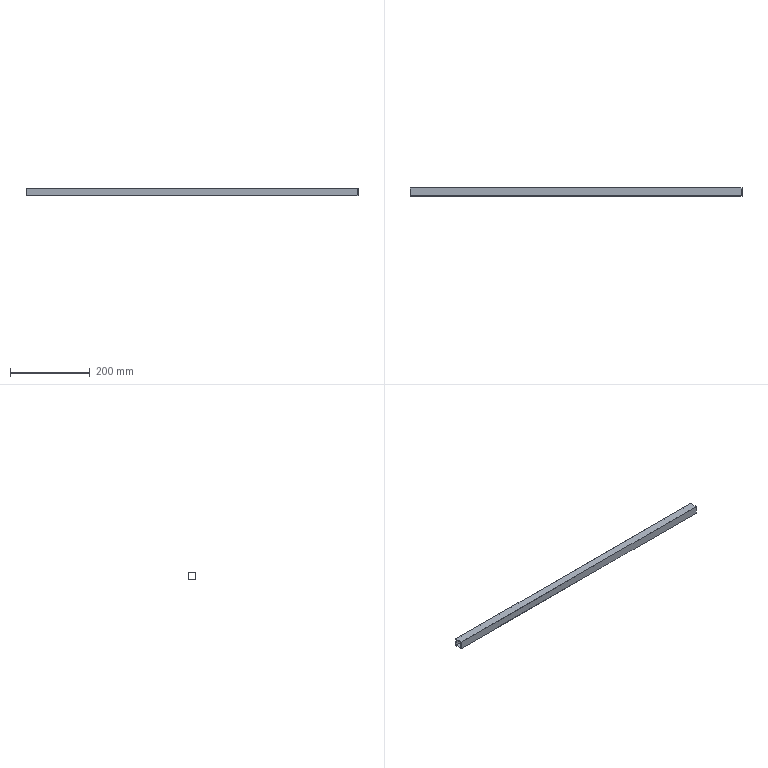Part | NX | features BREP 1 | 1 solid | 10 faces | box 830.914 x 20 x 20 mm | volume 119652 mm3 | plane 10
STEP:
#1=CARTESIAN_POINT('',(1608.587,-696.,89.999));
#2=VERTEX_POINT('',#1);
#3=CARTESIAN_POINT('',(1608.587,-680.,89.999));
#4=VERTEX_POINT('',#3);
#5=CARTESIAN_POINT('',(1608.587,-688.,89.999));
#6=DIRECTION('',(0.,1.,0.));
#7=VECTOR('',#6,1000.);
#8=LINE('',#5,#7);
#9=EDGE_CURVE('',#2,#4,#8,.T.);
#10=ORIENTED_EDGE('',*,*,#9,.F.);
#11=CARTESIAN_POINT('',(1608.587,-696.,105.999));
#12=VERTEX_POINT('',#11);
#13=CARTESIAN_POINT('',(1608.587,-696.,97.999));
#14=DIRECTION('',(0.,0.,1.));
#15=VECTOR('',#14,1000.);
#16=LINE('',#13,#15);
#17=EDGE_CURVE('',#2,#12,#16,.T.);
#18=ORIENTED_EDGE('',*,*,#17,.T.);
#19=CARTESIAN_POINT('',(1608.587,-680.,105.999));
#20=VERTEX_POINT('',#19);
#21=CARTESIAN_POINT('',(1608.587,-688.,105.999));
#22=DIRECTION('',(0.,-1.,0.));
#23=VECTOR('',#22,1000.);
#24=LINE('',#21,#23);
#25=EDGE_CURVE('',#20,#12,#24,.T.);
#26=ORIENTED_EDGE('',*,*,#25,.F.);
#27=CARTESIAN_POINT('',(1608.587,-680.,97.999));
#28=DIRECTION('',(0.,0.,1.));
#29=VECTOR('',#28,1000.);
#30=LINE('',#27,#29);
#31=EDGE_CURVE('',#4,#20,#30,.T.);
#32=ORIENTED_EDGE('',*,*,#31,.F.);
#33=EDGE_LOOP('',(#10,#18,#26,#32));
#34=FACE_BOUND('',#33,.T.);
#35=CARTESIAN_POINT('',(1608.587,-698.,87.999));
#36=VERTEX_POINT('',#35);
#37=CARTESIAN_POINT('',(1608.587,-698.,107.999));
#38=VERTEX_POINT('',#37);
#39=CARTESIAN_POINT('',(1608.587,-698.,87.999));
#40=CARTESIAN_POINT('',(1608.587,-698.,107.999));
#41=B_SPLINE_CURVE_WITH_KNOTS('',1,(#39,#40),.UNSPECIFIED.,.F.,.F.,(2,2),(0.,20.),.UNSPECIFIED.);
#42=EDGE_CURVE('',#36,#38,#41,.T.);
#43=ORIENTED_EDGE('',*,*,#42,.F.);
#44=CARTESIAN_POINT('',(1608.587,-678.,87.999));
#45=VERTEX_POINT('',#44);
#46=CARTESIAN_POINT('',(1608.587,-688.,87.999));
#47=DIRECTION('',(0.,1.,0.));
#48=VECTOR('',#47,1000.);
#49=LINE('',#46,#48);
#50=EDGE_CURVE('',#36,#45,#49,.T.);
#51=ORIENTED_EDGE('',*,*,#50,.T.);
#52=CARTESIAN_POINT('',(1608.587,-678.,107.999));
#53=VERTEX_POINT('',#52);
#54=CARTESIAN_POINT('',(1608.587,-678.,97.999));
#55=DIRECTION('',(0.,0.,1.));
#56=VECTOR('',#55,1000.);
#57=LINE('',#54,#56);
#58=EDGE_CURVE('',#45,#53,#57,.T.);
#59=ORIENTED_EDGE('',*,*,#58,.T.);
#60=CARTESIAN_POINT('',(1608.587,-688.,107.999));
#61=DIRECTION('',(0.,-1.,0.));
#62=VECTOR('',#61,1000.);
#63=LINE('',#60,#62);
#64=EDGE_CURVE('',#53,#38,#63,.T.);
#65=ORIENTED_EDGE('',*,*,#64,.T.);
#66=EDGE_LOOP('',(#43,#51,#59,#65));
#67=FACE_BOUND('',#66,.T.);
#68=CARTESIAN_POINT('',(1608.587,-688.,659.408));
#69=DIRECTION('',(1.,0.,0.));
#70=DIRECTION('',(0.,0.,-1.));
#71=AXIS2_PLACEMENT_3D('',#68,#69,#70);
#72=PLANE('',#71);
#73=ADVANCED_FACE('',(#34,#67),#72,.T.);
#74=CARTESIAN_POINT('',(777.673,-680.,105.999));
#75=VERTEX_POINT('',#74);
#76=CARTESIAN_POINT('',(1193.13,-680.,105.999));
#77=DIRECTION('',(1.,0.,0.));
#78=VECTOR('',#77,1000.);
#79=LINE('',#76,#78);
#80=EDGE_CURVE('',#75,#20,#79,.T.);
#81=ORIENTED_EDGE('',*,*,#80,.F.);
#82=CARTESIAN_POINT('',(777.673,-680.,89.999));
#83=VERTEX_POINT('',#82);
#84=CARTESIAN_POINT('',(777.673,-680.,89.999));
#85=CARTESIAN_POINT('',(777.673,-680.,93.199));
#86=CARTESIAN_POINT('',(777.673,-680.,96.399));
#87=CARTESIAN_POINT('',(777.673,-680.,99.599));
#88=CARTESIAN_POINT('',(777.673,-680.,102.799));
#89=CARTESIAN_POINT('',(777.673,-680.,105.999));
#90=B_SPLINE_CURVE_WITH_KNOTS('',5,(#84,#85,#86,#87,#88,#89),.UNSPECIFIED.,.F.,.F.,(6,6),(-286.004,-270.004),.UNSPECIFIED.);
#91=EDGE_CURVE('',#83,#75,#90,.T.);
#92=ORIENTED_EDGE('',*,*,#91,.F.);
#93=CARTESIAN_POINT('',(1193.13,-680.,89.999));
#94=DIRECTION('',(1.,0.,0.));
#95=VECTOR('',#94,1000.);
#96=LINE('',#93,#95);
#97=EDGE_CURVE('',#83,#4,#96,.T.);
#98=ORIENTED_EDGE('',*,*,#97,.T.);
#99=ORIENTED_EDGE('',*,*,#31,.T.);
#100=EDGE_LOOP('',(#81,#92,#98,#99));
#101=FACE_BOUND('',#100,.T.);
#102=CARTESIAN_POINT('',(687.53,-680.,87.999));
#103=DIRECTION('',(0.,-1.,0.));
#104=DIRECTION('',(1.,0.,0.));
#105=AXIS2_PLACEMENT_3D('',#102,#103,#104);
#106=PLANE('',#105);
#107=ADVANCED_FACE('',(#101),#106,.T.);
#108=ORIENTED_EDGE('',*,*,#97,.F.);
#109=CARTESIAN_POINT('',(777.673,-696.,89.999));
#110=VERTEX_POINT('',#109);
#111=CARTESIAN_POINT('',(777.673,-696.,89.999));
#112=CARTESIAN_POINT('',(777.673,-692.8,89.999));
#113=CARTESIAN_POINT('',(777.673,-689.6,89.999));
#114=CARTESIAN_POINT('',(777.673,-686.4,89.999));
#115=CARTESIAN_POINT('',(777.673,-683.2,89.999));
#116=CARTESIAN_POINT('',(777.673,-680.,89.999));
#117=B_SPLINE_CURVE_WITH_KNOTS('',5,(#111,#112,#113,#114,#115,#116),.UNSPECIFIED.,.F.,.F.,(6,6),(2.,18.),.UNSPECIFIED.);
#118=EDGE_CURVE('',#110,#83,#117,.T.);
#119=ORIENTED_EDGE('',*,*,#118,.F.);
#120=CARTESIAN_POINT('',(1193.13,-696.,89.999));
#121=DIRECTION('',(1.,0.,0.));
#122=VECTOR('',#121,1000.);
#123=LINE('',#120,#122);
#124=EDGE_CURVE('',#110,#2,#123,.T.);
#125=ORIENTED_EDGE('',*,*,#124,.T.);
#126=ORIENTED_EDGE('',*,*,#9,.T.);
#127=EDGE_LOOP('',(#108,#119,#125,#126));
#128=FACE_BOUND('',#127,.T.);
#129=CARTESIAN_POINT('',(687.53,-698.,89.999));
#130=DIRECTION('',(0.,0.,1.));
#131=DIRECTION('',(1.,0.,0.));
#132=AXIS2_PLACEMENT_3D('',#129,#130,#131);
#133=PLANE('',#132);
#134=ADVANCED_FACE('',(#128),#133,.T.);
#135=ORIENTED_EDGE('',*,*,#17,.F.);
#136=ORIENTED_EDGE('',*,*,#124,.F.);
#137=CARTESIAN_POINT('',(777.673,-696.,105.999));
#138=VERTEX_POINT('',#137);
#139=CARTESIAN_POINT('',(777.673,-696.,89.999));
#140=CARTESIAN_POINT('',(777.673,-696.,93.199));
#141=CARTESIAN_POINT('',(777.673,-696.,96.399));
#142=CARTESIAN_POINT('',(777.673,-696.,99.599));
#143=CARTESIAN_POINT('',(777.673,-696.,102.799));
#144=CARTESIAN_POINT('',(777.673,-696.,105.999));
#145=B_SPLINE_CURVE_WITH_KNOTS('',5,(#139,#140,#141,#142,#143,#144),.UNSPECIFIED.,.F.,.F.,(6,6),(-286.004,-270.004),.UNSPECIFIED.);
#146=EDGE_CURVE('',#110,#138,#145,.T.);
#147=ORIENTED_EDGE('',*,*,#146,.T.);
#148=CARTESIAN_POINT('',(1193.13,-696.,105.999));
#149=DIRECTION('',(1.,0.,0.));
#150=VECTOR('',#149,1000.);
#151=LINE('',#148,#150);
#152=EDGE_CURVE('',#138,#12,#151,.T.);
#153=ORIENTED_EDGE('',*,*,#152,.T.);
#154=EDGE_LOOP('',(#135,#136,#147,#153));
#155=FACE_BOUND('',#154,.T.);
#156=CARTESIAN_POINT('',(777.673,-696.,89.999));
#157=DIRECTION('',(0.,-1.,0.));
#158=DIRECTION('',(1.,0.,0.));
#159=AXIS2_PLACEMENT_3D('',#156,#157,#158);
#160=PLANE('',#159);
#161=ADVANCED_FACE('',(#155),#160,.F.);
#162=ORIENTED_EDGE('',*,*,#152,.F.);
#163=CARTESIAN_POINT('',(777.673,-696.,105.999));
#164=CARTESIAN_POINT('',(777.673,-692.8,105.999));
#165=CARTESIAN_POINT('',(777.673,-689.6,105.999));
#166=CARTESIAN_POINT('',(777.673,-686.4,105.999));
#167=CARTESIAN_POINT('',(777.673,-683.2,105.999));
#168=CARTESIAN_POINT('',(777.673,-680.,105.999));
#169=B_SPLINE_CURVE_WITH_KNOTS('',5,(#163,#164,#165,#166,#167,#168),.UNSPECIFIED.,.F.,.F.,(6,6),(2.,18.),.UNSPECIFIED.);
#170=EDGE_CURVE('',#138,#75,#169,.T.);
#171=ORIENTED_EDGE('',*,*,#170,.T.);
#172=ORIENTED_EDGE('',*,*,#80,.T.);
#173=ORIENTED_EDGE('',*,*,#25,.T.);
#174=EDGE_LOOP('',(#162,#171,#172,#173));
#175=FACE_BOUND('',#174,.T.);
#176=CARTESIAN_POINT('',(687.53,-678.,105.999));
#177=DIRECTION('',(0.,0.,-1.));
#178=DIRECTION('',(1.,0.,0.));
#179=AXIS2_PLACEMENT_3D('',#176,#177,#178);
#180=PLANE('',#179);
#181=ADVANCED_FACE('',(#175),#180,.T.);
#182=ORIENTED_EDGE('',*,*,#64,.F.);
#183=CARTESIAN_POINT('',(777.673,-678.,107.999));
#184=VERTEX_POINT('',#183);
#185=CARTESIAN_POINT('',(1193.13,-678.,107.999));
#186=DIRECTION('',(-1.,0.,0.));
#187=VECTOR('',#186,1000.);
#188=LINE('',#185,#187);
#189=EDGE_CURVE('',#53,#184,#188,.T.);
#190=ORIENTED_EDGE('',*,*,#189,.T.);
#191=CARTESIAN_POINT('',(777.673,-698.,107.999));
#192=VERTEX_POINT('',#191);
#193=CARTESIAN_POINT('',(777.673,-698.,107.999));
#194=CARTESIAN_POINT('',(777.673,-694.,107.999));
#195=CARTESIAN_POINT('',(777.673,-690.,107.999));
#196=CARTESIAN_POINT('',(777.673,-686.,107.999));
#197=CARTESIAN_POINT('',(777.673,-682.,107.999));
#198=CARTESIAN_POINT('',(777.673,-678.,107.999));
#199=B_SPLINE_CURVE_WITH_KNOTS('',5,(#193,#194,#195,#196,#197,#198),.UNSPECIFIED.,.F.,.F.,(6,6),(0.,20.),.UNSPECIFIED.);
#200=EDGE_CURVE('',#192,#184,#199,.T.);
#201=ORIENTED_EDGE('',*,*,#200,.F.);
#202=CARTESIAN_POINT('',(777.673,-698.,107.999));
#203=CARTESIAN_POINT('',(943.856,-698.,107.999));
#204=CARTESIAN_POINT('',(1110.039,-698.,107.999));
#205=CARTESIAN_POINT('',(1276.222,-698.,107.999));
#206=CARTESIAN_POINT('',(1442.405,-698.,107.999));
#207=CARTESIAN_POINT('',(1608.587,-698.,107.999));
#208=B_SPLINE_CURVE_WITH_KNOTS('',5,(#202,#203,#204,#205,#206,#207),.UNSPECIFIED.,.F.,.F.,(6,6),(90.143,921.057),.UNSPECIFIED.);
#209=EDGE_CURVE('',#192,#38,#208,.T.);
#210=ORIENTED_EDGE('',*,*,#209,.T.);
#211=EDGE_LOOP('',(#182,#190,#201,#210));
#212=FACE_BOUND('',#211,.T.);
#213=CARTESIAN_POINT('',(687.53,-678.,107.999));
#214=DIRECTION('',(0.,0.,-1.));
#215=DIRECTION('',(1.,0.,0.));
#216=AXIS2_PLACEMENT_3D('',#213,#214,#215);
#217=PLANE('',#216);
#218=ADVANCED_FACE('',(#212),#217,.F.);
#219=ORIENTED_EDGE('',*,*,#209,.F.);
#220=CARTESIAN_POINT('',(777.673,-698.,87.999));
#221=VERTEX_POINT('',#220);
#222=CARTESIAN_POINT('',(777.673,-698.,87.999));
#223=CARTESIAN_POINT('',(777.673,-698.,91.999));
#224=CARTESIAN_POINT('',(777.673,-698.,95.999));
#225=CARTESIAN_POINT('',(777.673,-698.,99.999));
#226=CARTESIAN_POINT('',(777.673,-698.,103.999));
#227=CARTESIAN_POINT('',(777.673,-698.,107.999));
#228=B_SPLINE_CURVE_WITH_KNOTS('',5,(#222,#223,#224,#225,#226,#227),.UNSPECIFIED.,.F.,.F.,(6,6),(-288.004,-268.004),.UNSPECIFIED.);
#229=EDGE_CURVE('',#221,#192,#228,.T.);
#230=ORIENTED_EDGE('',*,*,#229,.F.);
#231=CARTESIAN_POINT('',(1193.13,-698.,87.999));
#232=DIRECTION('',(1.,0.,0.));
#233=VECTOR('',#232,1000.);
#234=LINE('',#231,#233);
#235=EDGE_CURVE('',#221,#36,#234,.T.);
#236=ORIENTED_EDGE('',*,*,#235,.T.);
#237=ORIENTED_EDGE('',*,*,#42,.T.);
#238=EDGE_LOOP('',(#219,#230,#236,#237));
#239=FACE_BOUND('',#238,.T.);
#240=CARTESIAN_POINT('',(1260.427,-698.,97.999));
#241=DIRECTION('',(0.,-1.,0.));
#242=DIRECTION('',(0.,0.,-1.));
#243=AXIS2_PLACEMENT_3D('',#240,#241,#242);
#244=PLANE('',#243);
#245=ADVANCED_FACE('',(#239),#244,.T.);
#246=ORIENTED_EDGE('',*,*,#50,.F.);
#247=ORIENTED_EDGE('',*,*,#235,.F.);
#248=CARTESIAN_POINT('',(777.673,-678.,87.999));
#249=VERTEX_POINT('',#248);
#250=CARTESIAN_POINT('',(777.673,-698.,87.999));
#251=CARTESIAN_POINT('',(777.673,-694.,87.999));
#252=CARTESIAN_POINT('',(777.673,-690.,87.999));
#253=CARTESIAN_POINT('',(777.673,-686.,87.999));
#254=CARTESIAN_POINT('',(777.673,-682.,87.999));
#255=CARTESIAN_POINT('',(777.673,-678.,87.999));
#256=B_SPLINE_CURVE_WITH_KNOTS('',5,(#250,#251,#252,#253,#254,#255),.UNSPECIFIED.,.F.,.F.,(6,6),(0.,20.),.UNSPECIFIED.);
#257=EDGE_CURVE('',#221,#249,#256,.T.);
#258=ORIENTED_EDGE('',*,*,#257,.T.);
#259=CARTESIAN_POINT('',(1193.13,-678.,87.999));
#260=DIRECTION('',(1.,0.,0.));
#261=VECTOR('',#260,1000.);
#262=LINE('',#259,#261);
#263=EDGE_CURVE('',#249,#45,#262,.T.);
#264=ORIENTED_EDGE('',*,*,#263,.T.);
#265=EDGE_LOOP('',(#246,#247,#258,#264));
#266=FACE_BOUND('',#265,.T.);
#267=CARTESIAN_POINT('',(687.53,-698.,87.999));
#268=DIRECTION('',(0.,0.,1.));
#269=DIRECTION('',(1.,0.,0.));
#270=AXIS2_PLACEMENT_3D('',#267,#268,#269);
#271=PLANE('',#270);
#272=ADVANCED_FACE('',(#266),#271,.F.);
#273=ORIENTED_EDGE('',*,*,#58,.F.);
#274=ORIENTED_EDGE('',*,*,#263,.F.);
#275=CARTESIAN_POINT('',(777.673,-678.,87.999));
#276=CARTESIAN_POINT('',(777.673,-678.,91.999));
#277=CARTESIAN_POINT('',(777.673,-678.,95.999));
#278=CARTESIAN_POINT('',(777.673,-678.,99.999));
#279=CARTESIAN_POINT('',(777.673,-678.,103.999));
#280=CARTESIAN_POINT('',(777.673,-678.,107.999));
#281=B_SPLINE_CURVE_WITH_KNOTS('',5,(#275,#276,#277,#278,#279,#280),.UNSPECIFIED.,.F.,.F.,(6,6),(-288.004,-268.004),.UNSPECIFIED.);
#282=EDGE_CURVE('',#249,#184,#281,.T.);
#283=ORIENTED_EDGE('',*,*,#282,.T.);
#284=ORIENTED_EDGE('',*,*,#189,.F.);
#285=EDGE_LOOP('',(#273,#274,#283,#284));
#286=FACE_BOUND('',#285,.T.);
#287=CARTESIAN_POINT('',(687.53,-678.,87.999));
#288=DIRECTION('',(0.,-1.,0.));
#289=DIRECTION('',(1.,0.,0.));
#290=AXIS2_PLACEMENT_3D('',#287,#288,#289);
#291=PLANE('',#290);
#292=ADVANCED_FACE('',(#286),#291,.F.);
#293=ORIENTED_EDGE('',*,*,#170,.F.);
#294=ORIENTED_EDGE('',*,*,#146,.F.);
#295=ORIENTED_EDGE('',*,*,#118,.T.);
#296=ORIENTED_EDGE('',*,*,#91,.T.);
#297=EDGE_LOOP('',(#293,#294,#295,#296));
#298=FACE_BOUND('',#297,.T.);
#299=ORIENTED_EDGE('',*,*,#282,.F.);
#300=ORIENTED_EDGE('',*,*,#257,.F.);
#301=ORIENTED_EDGE('',*,*,#229,.T.);
#302=ORIENTED_EDGE('',*,*,#200,.T.);
#303=EDGE_LOOP('',(#299,#300,#301,#302));
#304=FACE_BOUND('',#303,.T.);
#305=CARTESIAN_POINT('',(777.673,-688.,593.034));
#306=DIRECTION('',(-1.,0.,0.));
#307=DIRECTION('',(0.,0.,1.));
#308=AXIS2_PLACEMENT_3D('',#305,#306,#307);
#309=PLANE('',#308);
#310=ADVANCED_FACE('',(#298,#304),#309,.T.);
#311=CLOSED_SHELL('',(#73,#107,#134,#161,#181,#218,#245,#272,#292,#310));
#312=MANIFOLD_SOLID_BREP('',#311);
#313=(LENGTH_UNIT()NAMED_UNIT(*)SI_UNIT(.MILLI.,.METRE.));
#314=UNCERTAINTY_MEASURE_WITH_UNIT(LENGTH_MEASURE(0.00001),#313,'','');
#315=(NAMED_UNIT(*)PLANE_ANGLE_UNIT()SI_UNIT($,.RADIAN.));
#316=(NAMED_UNIT(*)SI_UNIT($,.STERADIAN.)SOLID_ANGLE_UNIT());
#317=(GEOMETRIC_REPRESENTATION_CONTEXT(3)GLOBAL_UNCERTAINTY_ASSIGNED_CONTEXT((#314))GLOBAL_UNIT_ASSIGNED_CONTEXT((#313,#315,#316))REPRESENTATION_CONTEXT('',''));
#318=ADVANCED_BREP_SHAPE_REPRESENTATION('',(#312),#317);